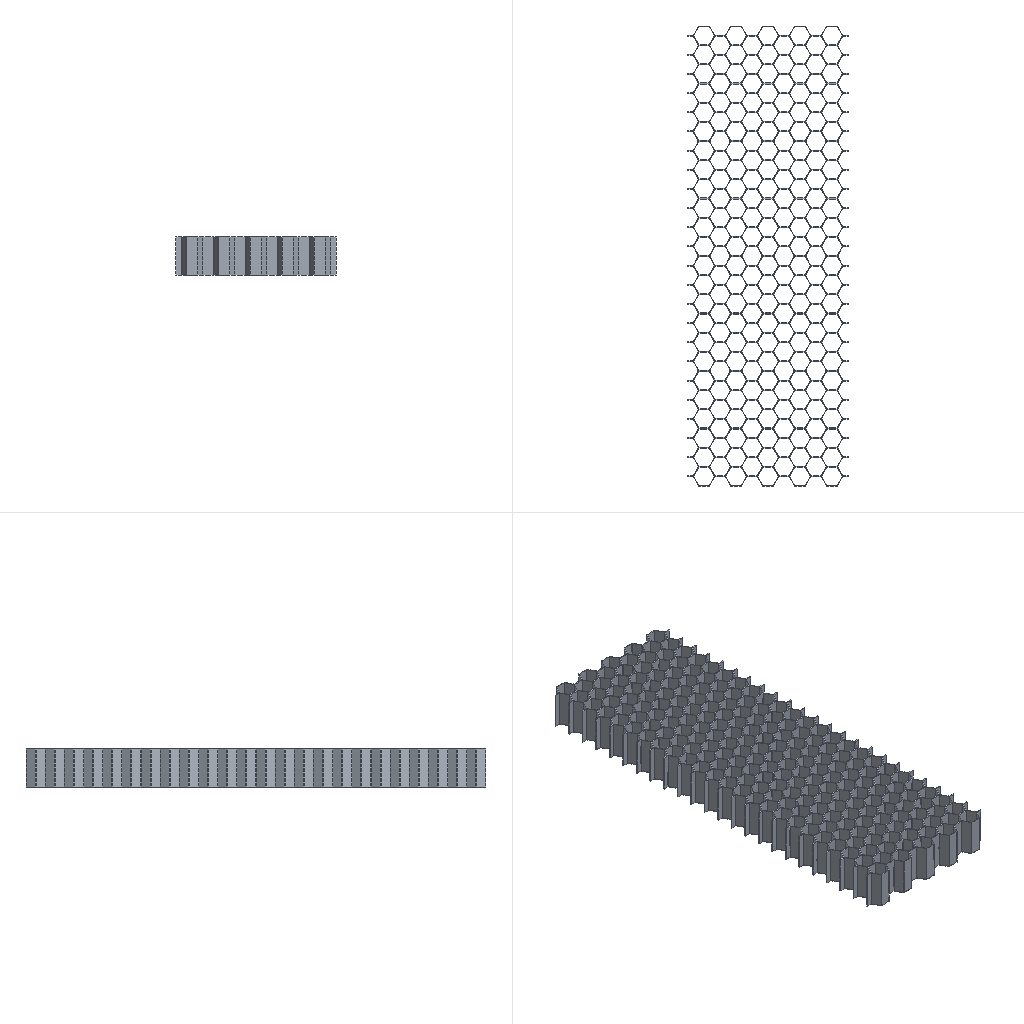Simulation study | abaqus
Set-up summary:
category,name,step,type,value,unit,region
solver,abaqus
solver,version,,,Abaqus/Explicit 2020
units,not stated in the deck,,not stated
analysis,deck,,transient,transient
load_step,Step-1,Step-1,transient,nlgeom=True
contact,interactions,,,general=1 pairs=0 ties=0
load_step,requested,,,1
mesh,nodes,,,77964
mesh,elements,,,78850
element_type,S3,,shell,940
element_type,S4R,,shell,47802
element_type,R3D4,,rigid,30108
load,load commands in deck,,count,2
bc,support commands in deck,,count,7
material,MATERIAL-1,,in results
check,setup vs results,,match,"per instance, exact: element labels, types and connectivity; labels of the nodes the elements use; coordinates of those nodes at SINGLE_PRECISION in 3 of 3 instance(s)"
Abaqus input file, long lists of numbers shortened:
*Heading
** Job name: Job-3 Model name: Model-3
** Generated by: Abaqus/CAE 2020
*Preprint, echo=NO, model=NO, history=NO, contact=NO
**
** PARTS
**
*Part, name=W-1
*Node
      1,  -20.784,  -55.51,   121.035
      2,  -22.234,  -55.51,   121.035
** (47848 more lines like these left out)
*Element, type=S4R
 1,    1,    2, 3093, 3110
 2, 3110, 3093, 3094, 3109
** (47800 more lines like these left out)
*Element, type=S3
43501, 1700,   14, 1688
43502, 1706, 1679, 1676
** (938 more lines like these left out)
*Nset, nset=Set-1, generate
     1,  47850,      1
*Elset, elset=Set-1, generate
     1,  48742,      1
** Section: Section-1
*Shell Section, elset=Set-1, material=Material-1
0.1, 5
*End Part
**
*Part, name=W-2
*Node
      1,   19.975,   62.868,   131.035
      2,  -22.235,   62.868,   131.035
** (15054 more lines like these left out)
*Element, type=R3D4
  1,    1,    9,  709,  118
  2,    9,   10,  710,  709
** (15052 more lines like these left out)
*Node
  15057,  -1.13,    2.348,   146.035
*Nset, nset=W-2-RefPt_, internal
15057,
*Elset, elset=W-2, generate
     1,  15054,      1
*End Part
**
*Part, name=W-3
*Node
      1,   19.975,   62.868,   106.035
      2,  -22.235,   62.868,   106.035
** (15054 more lines like these left out)
*Element, type=R3D4
  1,    1,    9,  709,  118
  2,    9,   10,  710,  709
** (15052 more lines like these left out)
*Node
  15057,  -1.13,    2.348,   121.035
*Nset, nset=W-3-RefPt_, internal
15057,
*Elset, elset=W-3, generate
     1,  15054,      1
*End Part
**
**
** ASSEMBLY
**
*Assembly, name=Assembly
**
*Instance, name=W-1-1, part=W-1
*End Instance
**
*Instance, name=W-2-1, part=W-2
*End Instance
**
*Instance, name=W-3-1, part=W-3
*End Instance
**
*Nset, nset=Set-1, instance=W-2-1
 15057,
*Nset, nset=Set-2, instance=W-3-1
 15057,
*Rigid Body, ref node=W-2-1.W-2-RefPt_, elset=W-2-1.W-2
*Rigid Body, ref node=W-3-1.W-3-RefPt_, elset=W-3-1.W-3
*End Assembly
*Amplitude, name=Amp-1
             0.,              0.,            0.01,              1.
**
** MATERIALS
**
*Material, name=Material-1
*Density
 1.8e-09,
*Elastic
16500., 0.35
**
** INTERACTION PROPERTIES
**
*Surface Interaction, name=IntProp-1
*Friction
 0.2,
*Surface Behavior, pressure-overclosure=HARD
** ----------------------------------------------------------------
**
** STEP: Step-1
**
*Step, name=Step-1, nlgeom=YES
*Dynamic, Explicit
, 0.01
*Bulk Viscosity
0.06, 1.2
** Mass Scaling: Semi-Automatic
**               Whole Model
*Fixed Mass Scaling, factor=5000.
**
** BOUNDARY CONDITIONS
**
** Name: BC-1 Type: 对称/反对称/完全固定
*Boundary
Set-1, ENCASTRE
** Name: [REDACTED] : Displacement/rotation angle
*Boundary, amplitude=Amp-1
Set-2, 1, 1
Set-2, 2, 2, -10.
Set-2, 3, 3, 0.1
Set-2, 4, 4
Set-2, 5, 5
Set-2, 6, 6
**
** INTERACTIONS
**
** Interaction: Int-1
*Contact, op=NEW
*Contact Inclusions, ALL EXTERIOR
*Contact Property Assignment
 ,  , IntProp-1
**
** OUTPUT REQUESTS
**
*Restart, write, number interval=1, time marks=NO
**
** FIELD OUTPUT: F-Output-1
**
*Output, field, number interval=30
*Node Output
A, CF, RF, RM, RT, U, V
*Element Output, directions=YES
E, EVF, LE, MISES, MISESMAX, MISESONLY, NE, PE, PEEQ, PEEQVAVG, PEVAVG, PRESSONLY, S, SEQUT, SF, SSAVG
SVAVG, YIELDPOT
*Contact Output
CDISP, CSTRESS
**
** HISTORY OUTPUT: H-Output-1
**
*Output, history, variable=PRESELECT
*End Step
Results summary:
result,step,Step-1,completed,increments=10009 time=0.01/0.01
result,analysis,,,transient
result,last_loadstep,,,1
result,analysis steps,,count,1
result,primary field,,,"U, UR"
result,reaction total,,FX,4084.682,model units
result,reaction total,,FY,-6296.875,model units
result,reaction total,,FZ,717.938,model units